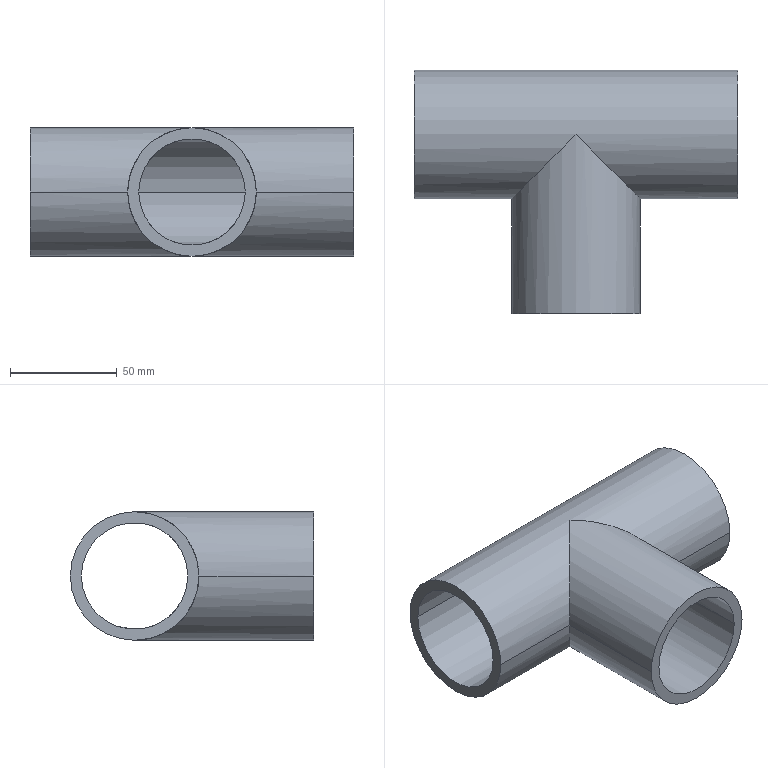Part | SolidWorks | features ICE 2, Sweep 2 | 1 solid | 15 faces | box 152 x 114.15 x 60.3 mm | volume 179160 mm3 | cylinder 10 | plane 5 | commonest cylinder face diameters 50 x6 60.3 x4
STEP:
#1=CARTESIAN_POINT('',(-76.,-25.,0.));
#2=VERTEX_POINT('',#1);
#3=CARTESIAN_POINT('',(-76.,25.,0.));
#4=VERTEX_POINT('',#3);
#5=CARTESIAN_POINT('',(-76.,0.,0.));
#6=DIRECTION('',(1.,0.,0.));
#7=DIRECTION('',(0.,1.,0.));
#8=AXIS2_PLACEMENT_3D('',#5,#6,#7);
#9=CIRCLE('',#8,25.);
#10=EDGE_CURVE('',#2,#4,#9,.T.);
#11=ORIENTED_EDGE('',*,*,#10,.F.);
#12=CARTESIAN_POINT('',(-25.,-25.,0.));
#13=VERTEX_POINT('',#12);
#14=CARTESIAN_POINT('',(-76.,-25.,0.));
#15=DIRECTION('',(1.,0.,0.));
#16=VECTOR('',#15,1000.);
#17=LINE('',#14,#16);
#18=EDGE_CURVE('',#2,#13,#17,.T.);
#19=ORIENTED_EDGE('',*,*,#18,.T.);
#20=CARTESIAN_POINT('',(0.,0.,-25.));
#21=VERTEX_POINT('',#20);
#22=CARTESIAN_POINT('',(-25.,-25.,0.));
#23=CARTESIAN_POINT('',(-25.,-25.,-14.645));
#24=CARTESIAN_POINT('',(-14.645,-14.645,-25.));
#25=CARTESIAN_POINT('',(0.,0.,-25.));
#26=(BOUNDED_CURVE()B_SPLINE_CURVE(3,(#22,#23,#24,#25),.UNSPECIFIED.,.F.,.F.)B_SPLINE_CURVE_WITH_KNOTS((4,4),(3.142,4.712),.UNSPECIFIED.)CURVE()GEOMETRIC_REPRESENTATION_ITEM()RATIONAL_B_SPLINE_CURVE((1.,0.8047,0.8047,1.))REPRESENTATION_ITEM(''));
#27=EDGE_CURVE('',#13,#21,#26,.T.);
#28=ORIENTED_EDGE('',*,*,#27,.T.);
#29=CARTESIAN_POINT('',(-1.,1.,-24.98));
#30=VERTEX_POINT('',#29);
#31=CARTESIAN_POINT('',(0.,0.,-25.));
#32=CARTESIAN_POINT('',(-0.3334,0.3334,-25.));
#33=CARTESIAN_POINT('',(-0.6668,0.6668,-24.993));
#34=CARTESIAN_POINT('',(-1.,1.,-24.98));
#35=(BOUNDED_CURVE()B_SPLINE_CURVE(3,(#31,#32,#33,#34),.UNSPECIFIED.,.F.,.F.)B_SPLINE_CURVE_WITH_KNOTS((4,4),(1.571,1.611),.UNSPECIFIED.)CURVE()GEOMETRIC_REPRESENTATION_ITEM()RATIONAL_B_SPLINE_CURVE((1.,0.9999,0.9999,1.))REPRESENTATION_ITEM(''));
#36=EDGE_CURVE('',#21,#30,#35,.T.);
#37=ORIENTED_EDGE('',*,*,#36,.T.);
#38=CARTESIAN_POINT('',(1.,1.,-24.98));
#39=VERTEX_POINT('',#38);
#40=CARTESIAN_POINT('',(-76.,1.,-24.98));
#41=DIRECTION('',(-1.,0.,0.));
#42=VECTOR('',#41,1000.);
#43=LINE('',#40,#42);
#44=EDGE_CURVE('',#39,#30,#43,.T.);
#45=ORIENTED_EDGE('',*,*,#44,.F.);
#46=CARTESIAN_POINT('',(1.,1.,-24.98));
#47=CARTESIAN_POINT('',(0.6668,0.6668,-24.993));
#48=CARTESIAN_POINT('',(0.3334,0.3334,-25.));
#49=CARTESIAN_POINT('',(0.,0.,-25.));
#50=(BOUNDED_CURVE()B_SPLINE_CURVE(3,(#46,#47,#48,#49),.UNSPECIFIED.,.F.,.F.)B_SPLINE_CURVE_WITH_KNOTS((4,4),(1.531,1.571),.UNSPECIFIED.)CURVE()GEOMETRIC_REPRESENTATION_ITEM()RATIONAL_B_SPLINE_CURVE((1.,0.9999,0.9999,1.))REPRESENTATION_ITEM(''));
#51=EDGE_CURVE('',#39,#21,#50,.T.);
#52=ORIENTED_EDGE('',*,*,#51,.T.);
#53=CARTESIAN_POINT('',(25.,-25.,0.));
#54=VERTEX_POINT('',#53);
#55=CARTESIAN_POINT('',(0.,0.,-25.));
#56=CARTESIAN_POINT('',(14.645,-14.645,-25.));
#57=CARTESIAN_POINT('',(25.,-25.,-14.645));
#58=CARTESIAN_POINT('',(25.,-25.,0.));
#59=(BOUNDED_CURVE()B_SPLINE_CURVE(3,(#55,#56,#57,#58),.UNSPECIFIED.,.F.,.F.)B_SPLINE_CURVE_WITH_KNOTS((4,4),(4.712,6.283),.UNSPECIFIED.)CURVE()GEOMETRIC_REPRESENTATION_ITEM()RATIONAL_B_SPLINE_CURVE((1.,0.8047,0.8047,1.))REPRESENTATION_ITEM(''));
#60=EDGE_CURVE('',#21,#54,#59,.T.);
#61=ORIENTED_EDGE('',*,*,#60,.T.);
#62=CARTESIAN_POINT('',(76.,-25.,0.));
#63=VERTEX_POINT('',#62);
#64=CARTESIAN_POINT('',(-76.,-25.,0.));
#65=DIRECTION('',(1.,0.,0.));
#66=VECTOR('',#65,1000.);
#67=LINE('',#64,#66);
#68=EDGE_CURVE('',#54,#63,#67,.T.);
#69=ORIENTED_EDGE('',*,*,#68,.T.);
#70=CARTESIAN_POINT('',(76.,25.,0.));
#71=VERTEX_POINT('',#70);
#72=CARTESIAN_POINT('',(76.,0.,0.));
#73=DIRECTION('',(1.,0.,0.));
#74=DIRECTION('',(0.,1.,0.));
#75=AXIS2_PLACEMENT_3D('',#72,#73,#74);
#76=CIRCLE('',#75,25.);
#77=EDGE_CURVE('',#63,#71,#76,.T.);
#78=ORIENTED_EDGE('',*,*,#77,.T.);
#79=CARTESIAN_POINT('',(-76.,25.,0.));
#80=DIRECTION('',(1.,0.,0.));
#81=VECTOR('',#80,1000.);
#82=LINE('',#79,#81);
#83=EDGE_CURVE('',#4,#71,#82,.T.);
#84=ORIENTED_EDGE('',*,*,#83,.F.);
#85=EDGE_LOOP('',(#11,#19,#28,#37,#45,#52,#61,#69,#78,#84));
#86=FACE_OUTER_BOUND('',#85,.T.);
#87=CARTESIAN_POINT('',(-76.,0.,0.));
#88=DIRECTION('',(1.,0.,0.));
#89=DIRECTION('',(0.,1.,0.));
#90=AXIS2_PLACEMENT_3D('',#87,#88,#89);
#91=CYLINDRICAL_SURFACE('',#90,25.);
#92=ADVANCED_FACE('',(#86),#91,.F.);
#93=ORIENTED_EDGE('',*,*,#27,.F.);
#94=CARTESIAN_POINT('',(-25.,-84.,0.));
#95=VERTEX_POINT('',#94);
#96=CARTESIAN_POINT('',(-25.,0.,0.));
#97=DIRECTION('',(0.,-1.,0.));
#98=VECTOR('',#97,1000.);
#99=LINE('',#96,#98);
#100=EDGE_CURVE('',#13,#95,#99,.T.);
#101=ORIENTED_EDGE('',*,*,#100,.T.);
#102=CARTESIAN_POINT('',(25.,-84.,0.));
#103=VERTEX_POINT('',#102);
#104=CARTESIAN_POINT('',(0.,-84.,0.));
#105=DIRECTION('',(0.,-1.,0.));
#106=DIRECTION('',(1.,0.,0.));
#107=AXIS2_PLACEMENT_3D('',#104,#105,#106);
#108=CIRCLE('',#107,25.);
#109=EDGE_CURVE('',#95,#103,#108,.T.);
#110=ORIENTED_EDGE('',*,*,#109,.T.);
#111=CARTESIAN_POINT('',(25.,0.,0.));
#112=DIRECTION('',(0.,-1.,0.));
#113=VECTOR('',#112,1000.);
#114=LINE('',#111,#113);
#115=EDGE_CURVE('',#54,#103,#114,.T.);
#116=ORIENTED_EDGE('',*,*,#115,.F.);
#117=ORIENTED_EDGE('',*,*,#60,.F.);
#118=EDGE_LOOP('',(#93,#101,#110,#116,#117));
#119=FACE_OUTER_BOUND('',#118,.T.);
#120=CARTESIAN_POINT('',(0.,0.,0.));
#121=DIRECTION('',(0.,-1.,0.));
#122=DIRECTION('',(1.,0.,0.));
#123=AXIS2_PLACEMENT_3D('',#120,#121,#122);
#124=CYLINDRICAL_SURFACE('',#123,25.);
#125=ADVANCED_FACE('',(#119),#124,.F.);
#126=CARTESIAN_POINT('',(0.,0.,30.15));
#127=VERTEX_POINT('',#126);
#128=CARTESIAN_POINT('',(-30.15,-30.15,0.));
#129=VERTEX_POINT('',#128);
#130=CARTESIAN_POINT('',(0.,0.,30.15));
#131=CARTESIAN_POINT('',(-17.661,-17.661,30.15));
#132=CARTESIAN_POINT('',(-30.15,-30.15,17.661));
#133=CARTESIAN_POINT('',(-30.15,-30.15,0.));
#134=(BOUNDED_CURVE()B_SPLINE_CURVE(3,(#130,#131,#132,#133),.UNSPECIFIED.,.F.,.F.)B_SPLINE_CURVE_WITH_KNOTS((4,4),(1.571,3.142),.UNSPECIFIED.)CURVE()GEOMETRIC_REPRESENTATION_ITEM()RATIONAL_B_SPLINE_CURVE((1.,0.8047,0.8047,1.))REPRESENTATION_ITEM(''));
#135=EDGE_CURVE('',#127,#129,#134,.T.);
#136=ORIENTED_EDGE('',*,*,#135,.T.);
#137=CARTESIAN_POINT('',(-30.15,-84.,0.));
#138=VERTEX_POINT('',#137);
#139=CARTESIAN_POINT('',(-30.15,0.,0.));
#140=DIRECTION('',(0.,-1.,0.));
#141=VECTOR('',#140,1000.);
#142=LINE('',#139,#141);
#143=EDGE_CURVE('',#129,#138,#142,.T.);
#144=ORIENTED_EDGE('',*,*,#143,.T.);
#145=CARTESIAN_POINT('',(30.15,-84.,0.));
#146=VERTEX_POINT('',#145);
#147=CARTESIAN_POINT('',(0.,-84.,0.));
#148=DIRECTION('',(0.,-1.,0.));
#149=DIRECTION('',(1.,0.,0.));
#150=AXIS2_PLACEMENT_3D('',#147,#148,#149);
#151=CIRCLE('',#150,30.15);
#152=EDGE_CURVE('',#146,#138,#151,.T.);
#153=ORIENTED_EDGE('',*,*,#152,.F.);
#154=CARTESIAN_POINT('',(30.15,-30.15,0.));
#155=VERTEX_POINT('',#154);
#156=CARTESIAN_POINT('',(30.15,0.,0.));
#157=DIRECTION('',(0.,-1.,0.));
#158=VECTOR('',#157,1000.);
#159=LINE('',#156,#158);
#160=EDGE_CURVE('',#155,#146,#159,.T.);
#161=ORIENTED_EDGE('',*,*,#160,.F.);
#162=CARTESIAN_POINT('',(30.15,-30.15,0.));
#163=CARTESIAN_POINT('',(30.15,-30.15,17.661));
#164=CARTESIAN_POINT('',(17.661,-17.661,30.15));
#165=CARTESIAN_POINT('',(0.,0.,30.15));
#166=(BOUNDED_CURVE()B_SPLINE_CURVE(3,(#162,#163,#164,#165),.UNSPECIFIED.,.F.,.F.)B_SPLINE_CURVE_WITH_KNOTS((4,4),(0.,1.571),.UNSPECIFIED.)CURVE()GEOMETRIC_REPRESENTATION_ITEM()RATIONAL_B_SPLINE_CURVE((1.,0.8047,0.8047,1.))REPRESENTATION_ITEM(''));
#167=EDGE_CURVE('',#155,#127,#166,.T.);
#168=ORIENTED_EDGE('',*,*,#167,.T.);
#169=EDGE_LOOP('',(#136,#144,#153,#161,#168));
#170=FACE_OUTER_BOUND('',#169,.T.);
#171=CARTESIAN_POINT('',(0.,0.,0.));
#172=DIRECTION('',(0.,-1.,0.));
#173=DIRECTION('',(1.,0.,0.));
#174=AXIS2_PLACEMENT_3D('',#171,#172,#173);
#175=CYLINDRICAL_SURFACE('',#174,30.15);
#176=ADVANCED_FACE('',(#170),#175,.T.);
#177=CARTESIAN_POINT('',(-76.,30.15,0.));
#178=VERTEX_POINT('',#177);
#179=CARTESIAN_POINT('',(-76.,-30.15,0.));
#180=VERTEX_POINT('',#179);
#181=CARTESIAN_POINT('',(-76.,0.,0.));
#182=DIRECTION('',(1.,0.,0.));
#183=DIRECTION('',(0.,1.,0.));
#184=AXIS2_PLACEMENT_3D('',#181,#182,#183);
#185=CIRCLE('',#184,30.15);
#186=EDGE_CURVE('',#178,#180,#185,.T.);
#187=ORIENTED_EDGE('',*,*,#186,.T.);
#188=CARTESIAN_POINT('',(-76.,-30.15,0.));
#189=DIRECTION('',(1.,0.,0.));
#190=VECTOR('',#189,1000.);
#191=LINE('',#188,#190);
#192=EDGE_CURVE('',#180,#129,#191,.T.);
#193=ORIENTED_EDGE('',*,*,#192,.T.);
#194=ORIENTED_EDGE('',*,*,#135,.F.);
#195=ORIENTED_EDGE('',*,*,#167,.F.);
#196=CARTESIAN_POINT('',(76.,-30.15,0.));
#197=VERTEX_POINT('',#196);
#198=CARTESIAN_POINT('',(-76.,-30.15,0.));
#199=DIRECTION('',(1.,0.,0.));
#200=VECTOR('',#199,1000.);
#201=LINE('',#198,#200);
#202=EDGE_CURVE('',#155,#197,#201,.T.);
#203=ORIENTED_EDGE('',*,*,#202,.T.);
#204=CARTESIAN_POINT('',(76.,30.15,0.));
#205=VERTEX_POINT('',#204);
#206=CARTESIAN_POINT('',(76.,0.,0.));
#207=DIRECTION('',(1.,0.,0.));
#208=DIRECTION('',(0.,1.,0.));
#209=AXIS2_PLACEMENT_3D('',#206,#207,#208);
#210=CIRCLE('',#209,30.15);
#211=EDGE_CURVE('',#205,#197,#210,.T.);
#212=ORIENTED_EDGE('',*,*,#211,.F.);
#213=CARTESIAN_POINT('',(-76.,30.15,0.));
#214=DIRECTION('',(1.,0.,0.));
#215=VECTOR('',#214,1000.);
#216=LINE('',#213,#215);
#217=EDGE_CURVE('',#178,#205,#216,.T.);
#218=ORIENTED_EDGE('',*,*,#217,.F.);
#219=EDGE_LOOP('',(#187,#193,#194,#195,#203,#212,#218));
#220=FACE_OUTER_BOUND('',#219,.T.);
#221=CARTESIAN_POINT('',(-76.,0.,0.));
#222=DIRECTION('',(1.,0.,0.));
#223=DIRECTION('',(0.,1.,0.));
#224=AXIS2_PLACEMENT_3D('',#221,#222,#223);
#225=CYLINDRICAL_SURFACE('',#224,30.15);
#226=ADVANCED_FACE('',(#220),#225,.T.);
#227=ORIENTED_EDGE('',*,*,#192,.F.);
#228=CARTESIAN_POINT('',(-76.,0.,0.));
#229=DIRECTION('',(1.,0.,0.));
#230=DIRECTION('',(0.,1.,0.));
#231=AXIS2_PLACEMENT_3D('',#228,#229,#230);
#232=CIRCLE('',#231,30.15);
#233=EDGE_CURVE('',#180,#178,#232,.T.);
#234=ORIENTED_EDGE('',*,*,#233,.T.);
#235=ORIENTED_EDGE('',*,*,#217,.T.);
#236=CARTESIAN_POINT('',(76.,0.,0.));
#237=DIRECTION('',(1.,0.,0.));
#238=DIRECTION('',(0.,1.,0.));
#239=AXIS2_PLACEMENT_3D('',#236,#237,#238);
#240=CIRCLE('',#239,30.15);
#241=EDGE_CURVE('',#197,#205,#240,.T.);
#242=ORIENTED_EDGE('',*,*,#241,.F.);
#243=ORIENTED_EDGE('',*,*,#202,.F.);
#244=CARTESIAN_POINT('',(0.,0.,-30.15));
#245=VERTEX_POINT('',#244);
#246=CARTESIAN_POINT('',(0.,0.,-30.15));
#247=CARTESIAN_POINT('',(17.661,-17.661,-30.15));
#248=CARTESIAN_POINT('',(30.15,-30.15,-17.661));
#249=CARTESIAN_POINT('',(30.15,-30.15,0.));
#250=(BOUNDED_CURVE()B_SPLINE_CURVE(3,(#246,#247,#248,#249),.UNSPECIFIED.,.F.,.F.)B_SPLINE_CURVE_WITH_KNOTS((4,4),(4.712,6.283),.UNSPECIFIED.)CURVE()GEOMETRIC_REPRESENTATION_ITEM()RATIONAL_B_SPLINE_CURVE((1.,0.8047,0.8047,1.))REPRESENTATION_ITEM(''));
#251=EDGE_CURVE('',#245,#155,#250,.T.);
#252=ORIENTED_EDGE('',*,*,#251,.F.);
#253=CARTESIAN_POINT('',(-30.15,-30.15,0.));
#254=CARTESIAN_POINT('',(-30.15,-30.15,-17.661));
#255=CARTESIAN_POINT('',(-17.661,-17.661,-30.15));
#256=CARTESIAN_POINT('',(0.,0.,-30.15));
#257=(BOUNDED_CURVE()B_SPLINE_CURVE(3,(#253,#254,#255,#256),.UNSPECIFIED.,.F.,.F.)B_SPLINE_CURVE_WITH_KNOTS((4,4),(3.142,4.712),.UNSPECIFIED.)CURVE()GEOMETRIC_REPRESENTATION_ITEM()RATIONAL_B_SPLINE_CURVE((1.,0.8047,0.8047,1.))REPRESENTATION_ITEM(''));
#258=EDGE_CURVE('',#129,#245,#257,.T.);
#259=ORIENTED_EDGE('',*,*,#258,.F.);
#260=EDGE_LOOP('',(#227,#234,#235,#242,#243,#252,#259));
#261=FACE_OUTER_BOUND('',#260,.T.);
#262=CARTESIAN_POINT('',(-76.,0.,0.));
#263=DIRECTION('',(1.,0.,0.));
#264=DIRECTION('',(0.,1.,0.));
#265=AXIS2_PLACEMENT_3D('',#262,#263,#264);
#266=CYLINDRICAL_SURFACE('',#265,30.15);
#267=ADVANCED_FACE('',(#261),#266,.T.);
#268=CARTESIAN_POINT('',(76.,0.,0.));
#269=DIRECTION('',(1.,0.,0.));
#270=DIRECTION('',(0.,1.,0.));
#271=AXIS2_PLACEMENT_3D('',#268,#269,#270);
#272=CIRCLE('',#271,25.);
#273=EDGE_CURVE('',#71,#63,#272,.T.);
#274=ORIENTED_EDGE('',*,*,#273,.F.);
#275=ORIENTED_EDGE('',*,*,#77,.F.);
#276=EDGE_LOOP('',(#274,#275));
#277=FACE_BOUND('',#276,.T.);
#278=ORIENTED_EDGE('',*,*,#211,.T.);
#279=ORIENTED_EDGE('',*,*,#241,.T.);
#280=EDGE_LOOP('',(#278,#279));
#281=FACE_OUTER_BOUND('',#280,.T.);
#282=CARTESIAN_POINT('',(76.,0.,0.));
#283=DIRECTION('',(1.,0.,0.));
#284=DIRECTION('',(0.,1.,0.));
#285=AXIS2_PLACEMENT_3D('',#282,#283,#284);
#286=PLANE('',#285);
#287=ADVANCED_FACE('',(#277,#281),#286,.T.);
#288=CARTESIAN_POINT('',(-76.,0.,0.));
#289=DIRECTION('',(1.,0.,0.));
#290=DIRECTION('',(0.,1.,0.));
#291=AXIS2_PLACEMENT_3D('',#288,#289,#290);
#292=CIRCLE('',#291,25.);
#293=EDGE_CURVE('',#4,#2,#292,.T.);
#294=ORIENTED_EDGE('',*,*,#293,.T.);
#295=ORIENTED_EDGE('',*,*,#10,.T.);
#296=EDGE_LOOP('',(#294,#295));
#297=FACE_BOUND('',#296,.T.);
#298=ORIENTED_EDGE('',*,*,#186,.F.);
#299=ORIENTED_EDGE('',*,*,#233,.F.);
#300=EDGE_LOOP('',(#298,#299));
#301=FACE_OUTER_BOUND('',#300,.T.);
#302=CARTESIAN_POINT('',(-76.,0.,0.));
#303=DIRECTION('',(1.,0.,0.));
#304=DIRECTION('',(0.,1.,0.));
#305=AXIS2_PLACEMENT_3D('',#302,#303,#304);
#306=PLANE('',#305);
#307=ADVANCED_FACE('',(#297,#301),#306,.F.);
#308=ORIENTED_EDGE('',*,*,#143,.F.);
#309=ORIENTED_EDGE('',*,*,#258,.T.);
#310=ORIENTED_EDGE('',*,*,#251,.T.);
#311=ORIENTED_EDGE('',*,*,#160,.T.);
#312=CARTESIAN_POINT('',(0.,-84.,0.));
#313=DIRECTION('',(0.,-1.,0.));
#314=DIRECTION('',(1.,0.,0.));
#315=AXIS2_PLACEMENT_3D('',#312,#313,#314);
#316=CIRCLE('',#315,30.15);
#317=EDGE_CURVE('',#138,#146,#316,.T.);
#318=ORIENTED_EDGE('',*,*,#317,.F.);
#319=EDGE_LOOP('',(#308,#309,#310,#311,#318));
#320=FACE_OUTER_BOUND('',#319,.T.);
#321=CARTESIAN_POINT('',(0.,0.,0.));
#322=DIRECTION('',(0.,-1.,0.));
#323=DIRECTION('',(1.,0.,0.));
#324=AXIS2_PLACEMENT_3D('',#321,#322,#323);
#325=CYLINDRICAL_SURFACE('',#324,30.15);
#326=ADVANCED_FACE('',(#320),#325,.T.);
#327=CARTESIAN_POINT('',(0.,-84.,0.));
#328=DIRECTION('',(0.,-1.,0.));
#329=DIRECTION('',(1.,0.,0.));
#330=AXIS2_PLACEMENT_3D('',#327,#328,#329);
#331=CIRCLE('',#330,25.);
#332=EDGE_CURVE('',#103,#95,#331,.T.);
#333=ORIENTED_EDGE('',*,*,#332,.F.);
#334=ORIENTED_EDGE('',*,*,#109,.F.);
#335=EDGE_LOOP('',(#333,#334));
#336=FACE_BOUND('',#335,.T.);
#337=ORIENTED_EDGE('',*,*,#152,.T.);
#338=ORIENTED_EDGE('',*,*,#317,.T.);
#339=EDGE_LOOP('',(#337,#338));
#340=FACE_OUTER_BOUND('',#339,.T.);
#341=CARTESIAN_POINT('',(0.,-84.,0.));
#342=DIRECTION('',(0.,-1.,0.));
#343=DIRECTION('',(1.,0.,0.));
#344=AXIS2_PLACEMENT_3D('',#341,#342,#343);
#345=PLANE('',#344);
#346=ADVANCED_FACE('',(#336,#340),#345,.T.);
#347=ORIENTED_EDGE('',*,*,#100,.F.);
#348=CARTESIAN_POINT('',(0.,0.,25.));
#349=VERTEX_POINT('',#348);
#350=CARTESIAN_POINT('',(0.,0.,25.));
#351=CARTESIAN_POINT('',(-14.645,-14.645,25.));
#352=CARTESIAN_POINT('',(-25.,-25.,14.645));
#353=CARTESIAN_POINT('',(-25.,-25.,0.));
#354=(BOUNDED_CURVE()B_SPLINE_CURVE(3,(#350,#351,#352,#353),.UNSPECIFIED.,.F.,.F.)B_SPLINE_CURVE_WITH_KNOTS((4,4),(1.571,3.142),.UNSPECIFIED.)CURVE()GEOMETRIC_REPRESENTATION_ITEM()RATIONAL_B_SPLINE_CURVE((1.,0.8047,0.8047,1.))REPRESENTATION_ITEM(''));
#355=EDGE_CURVE('',#349,#13,#354,.T.);
#356=ORIENTED_EDGE('',*,*,#355,.F.);
#357=CARTESIAN_POINT('',(25.,-25.,0.));
#358=CARTESIAN_POINT('',(25.,-25.,14.645));
#359=CARTESIAN_POINT('',(14.645,-14.645,25.));
#360=CARTESIAN_POINT('',(0.,0.,25.));
#361=(BOUNDED_CURVE()B_SPLINE_CURVE(3,(#357,#358,#359,#360),.UNSPECIFIED.,.F.,.F.)B_SPLINE_CURVE_WITH_KNOTS((4,4),(0.,1.571),.UNSPECIFIED.)CURVE()GEOMETRIC_REPRESENTATION_ITEM()RATIONAL_B_SPLINE_CURVE((1.,0.8047,0.8047,1.))REPRESENTATION_ITEM(''));
#362=EDGE_CURVE('',#54,#349,#361,.T.);
#363=ORIENTED_EDGE('',*,*,#362,.F.);
#364=ORIENTED_EDGE('',*,*,#115,.T.);
#365=ORIENTED_EDGE('',*,*,#332,.T.);
#366=EDGE_LOOP('',(#347,#356,#363,#364,#365));
#367=FACE_OUTER_BOUND('',#366,.T.);
#368=CARTESIAN_POINT('',(0.,0.,0.));
#369=DIRECTION('',(0.,-1.,0.));
#370=DIRECTION('',(1.,0.,0.));
#371=AXIS2_PLACEMENT_3D('',#368,#369,#370);
#372=CYLINDRICAL_SURFACE('',#371,25.);
#373=ADVANCED_FACE('',(#367),#372,.F.);
#374=ORIENTED_EDGE('',*,*,#18,.F.);
#375=ORIENTED_EDGE('',*,*,#293,.F.);
#376=ORIENTED_EDGE('',*,*,#83,.T.);
#377=ORIENTED_EDGE('',*,*,#273,.T.);
#378=ORIENTED_EDGE('',*,*,#68,.F.);
#379=ORIENTED_EDGE('',*,*,#362,.T.);
#380=CARTESIAN_POINT('',(1.,1.,24.98));
#381=VERTEX_POINT('',#380);
#382=CARTESIAN_POINT('',(0.,0.,25.));
#383=CARTESIAN_POINT('',(0.3334,0.3334,25.));
#384=CARTESIAN_POINT('',(0.6668,0.6668,24.993));
#385=CARTESIAN_POINT('',(1.,1.,24.98));
#386=(BOUNDED_CURVE()B_SPLINE_CURVE(3,(#382,#383,#384,#385),.UNSPECIFIED.,.F.,.F.)B_SPLINE_CURVE_WITH_KNOTS((4,4),(4.712,4.752),.UNSPECIFIED.)CURVE()GEOMETRIC_REPRESENTATION_ITEM()RATIONAL_B_SPLINE_CURVE((1.,0.9999,0.9999,1.))REPRESENTATION_ITEM(''));
#387=EDGE_CURVE('',#349,#381,#386,.T.);
#388=ORIENTED_EDGE('',*,*,#387,.T.);
#389=CARTESIAN_POINT('',(-1.,1.,24.98));
#390=VERTEX_POINT('',#389);
#391=CARTESIAN_POINT('',(-76.,1.,24.98));
#392=DIRECTION('',(1.,0.,0.));
#393=VECTOR('',#392,1000.);
#394=LINE('',#391,#393);
#395=EDGE_CURVE('',#390,#381,#394,.T.);
#396=ORIENTED_EDGE('',*,*,#395,.F.);
#397=CARTESIAN_POINT('',(-1.,1.,24.98));
#398=CARTESIAN_POINT('',(-0.6668,0.6668,24.993));
#399=CARTESIAN_POINT('',(-0.3334,0.3334,25.));
#400=CARTESIAN_POINT('',(0.,0.,25.));
#401=(BOUNDED_CURVE()B_SPLINE_CURVE(3,(#397,#398,#399,#400),.UNSPECIFIED.,.F.,.F.)B_SPLINE_CURVE_WITH_KNOTS((4,4),(4.672,4.712),.UNSPECIFIED.)CURVE()GEOMETRIC_REPRESENTATION_ITEM()RATIONAL_B_SPLINE_CURVE((1.,0.9999,0.9999,1.))REPRESENTATION_ITEM(''));
#402=EDGE_CURVE('',#390,#349,#401,.T.);
#403=ORIENTED_EDGE('',*,*,#402,.T.);
#404=ORIENTED_EDGE('',*,*,#355,.T.);
#405=EDGE_LOOP('',(#374,#375,#376,#377,#378,#379,#388,#396,#403,#404));
#406=FACE_OUTER_BOUND('',#405,.T.);
#407=CARTESIAN_POINT('',(-76.,0.,0.));
#408=DIRECTION('',(1.,0.,0.));
#409=DIRECTION('',(0.,1.,0.));
#410=AXIS2_PLACEMENT_3D('',#407,#408,#409);
#411=CYLINDRICAL_SURFACE('',#410,25.);
#412=ADVANCED_FACE('',(#406),#411,.F.);
#413=ORIENTED_EDGE('',*,*,#395,.T.);
#414=CARTESIAN_POINT('',(0.,1.,0.));
#415=DIRECTION('',(0.,-1.,0.));
#416=DIRECTION('',(1.,0.,0.));
#417=AXIS2_PLACEMENT_3D('',#414,#415,#416);
#418=CIRCLE('',#417,25.);
#419=EDGE_CURVE('',#381,#390,#418,.T.);
#420=ORIENTED_EDGE('',*,*,#419,.T.);
#421=EDGE_LOOP('',(#413,#420));
#422=FACE_OUTER_BOUND('',#421,.T.);
#423=CARTESIAN_POINT('',(0.,1.,0.));
#424=DIRECTION('',(0.,-1.,0.));
#425=DIRECTION('',(1.,0.,0.));
#426=AXIS2_PLACEMENT_3D('',#423,#424,#425);
#427=PLANE('',#426);
#428=ADVANCED_FACE('',(#422),#427,.T.);
#429=ORIENTED_EDGE('',*,*,#402,.F.);
#430=ORIENTED_EDGE('',*,*,#419,.F.);
#431=ORIENTED_EDGE('',*,*,#387,.F.);
#432=EDGE_LOOP('',(#429,#430,#431));
#433=FACE_OUTER_BOUND('',#432,.T.);
#434=CARTESIAN_POINT('',(0.,1.,0.));
#435=DIRECTION('',(0.,-1.,0.));
#436=DIRECTION('',(1.,0.,0.));
#437=AXIS2_PLACEMENT_3D('',#434,#435,#436);
#438=CYLINDRICAL_SURFACE('',#437,25.);
#439=ADVANCED_FACE('',(#433),#438,.F.);
#440=ORIENTED_EDGE('',*,*,#44,.T.);
#441=CARTESIAN_POINT('',(0.,1.,0.));
#442=DIRECTION('',(0.,-1.,0.));
#443=DIRECTION('',(1.,0.,0.));
#444=AXIS2_PLACEMENT_3D('',#441,#442,#443);
#445=CIRCLE('',#444,25.);
#446=EDGE_CURVE('',#30,#39,#445,.T.);
#447=ORIENTED_EDGE('',*,*,#446,.T.);
#448=EDGE_LOOP('',(#440,#447));
#449=FACE_OUTER_BOUND('',#448,.T.);
#450=CARTESIAN_POINT('',(0.,1.,0.));
#451=DIRECTION('',(0.,-1.,0.));
#452=DIRECTION('',(1.,0.,0.));
#453=AXIS2_PLACEMENT_3D('',#450,#451,#452);
#454=PLANE('',#453);
#455=ADVANCED_FACE('',(#449),#454,.T.);
#456=ORIENTED_EDGE('',*,*,#446,.F.);
#457=ORIENTED_EDGE('',*,*,#36,.F.);
#458=ORIENTED_EDGE('',*,*,#51,.F.);
#459=EDGE_LOOP('',(#456,#457,#458));
#460=FACE_OUTER_BOUND('',#459,.T.);
#461=CARTESIAN_POINT('',(0.,1.,0.));
#462=DIRECTION('',(0.,-1.,0.));
#463=DIRECTION('',(1.,0.,0.));
#464=AXIS2_PLACEMENT_3D('',#461,#462,#463);
#465=CYLINDRICAL_SURFACE('',#464,25.);
#466=ADVANCED_FACE('',(#460),#465,.F.);
#467=CLOSED_SHELL('',(#92,#125,#176,#226,#267,#287,#307,#326,#346,#373,#412,#428,#439,#455,#466));
#468=MANIFOLD_SOLID_BREP('',#467);
#469=CARTESIAN_POINT('',(0.,0.,0.));
#470=DIRECTION('',(0.,0.,1.));
#471=DIRECTION('',(1.,0.,0.));
#472=AXIS2_PLACEMENT_3D('',#469,#470,#471);
#473=(LENGTH_UNIT()NAMED_UNIT(*)SI_UNIT(.MILLI.,.METRE.));
#474=UNCERTAINTY_MEASURE_WITH_UNIT(LENGTH_MEASURE(0.00001),#473,'','');
#475=(NAMED_UNIT(*)PLANE_ANGLE_UNIT()SI_UNIT($,.RADIAN.));
#476=(NAMED_UNIT(*)SI_UNIT($,.STERADIAN.)SOLID_ANGLE_UNIT());
#477=(GEOMETRIC_REPRESENTATION_CONTEXT(3)GLOBAL_UNCERTAINTY_ASSIGNED_CONTEXT((#474))GLOBAL_UNIT_ASSIGNED_CONTEXT((#473,#475,#476))REPRESENTATION_CONTEXT('',''));
#478=ADVANCED_BREP_SHAPE_REPRESENTATION('',(#468,#472),#477);